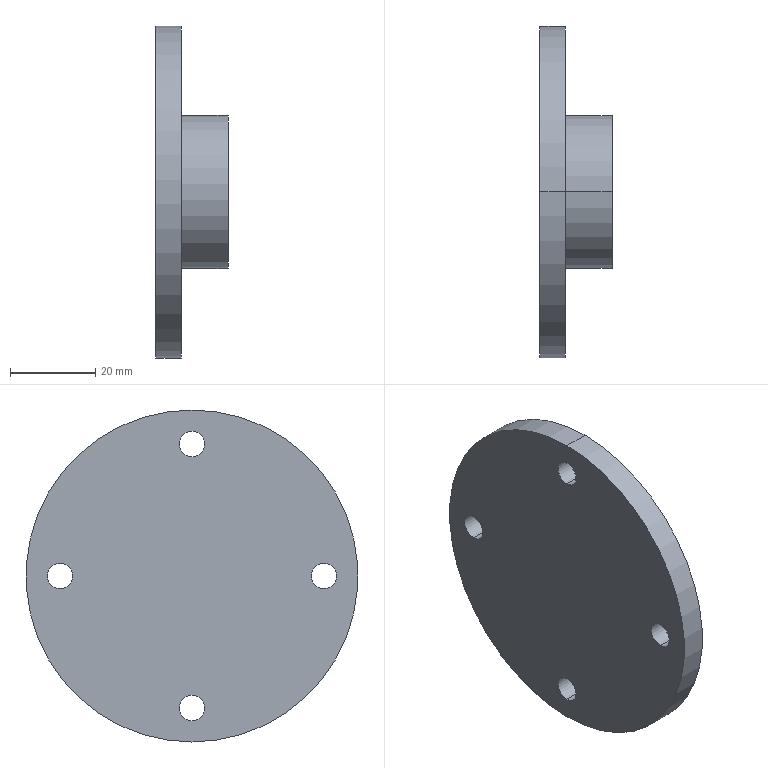Part | NX | features BREP 1 | 1 solid | 18 faces | box 17 x 78 x 78 mm | volume 32864 mm3 | cylinder 12 | plane 4 | cone 2 | commonest cylinder face diameters 6 x8 36 x2 78 x2
STEP:
#1=CARTESIAN_POINT('',(6.,0.,-28.));
#2=VERTEX_POINT('',#1);
#3=CARTESIAN_POINT('',(6.,0.,-34.));
#4=VERTEX_POINT('',#3);
#5=CARTESIAN_POINT('',(6.,0.,-31.));
#6=DIRECTION('',(1.,0.,0.));
#7=DIRECTION('',(0.,0.,1.));
#8=AXIS2_PLACEMENT_3D('',#5,#6,#7);
#9=CIRCLE('',#8,3.);
#10=EDGE_CURVE('',#2,#4,#9,.T.);
#11=ORIENTED_EDGE('',*,*,#10,.T.);
#12=CARTESIAN_POINT('',(0.,0.,-34.));
#13=VERTEX_POINT('',#12);
#14=CARTESIAN_POINT('',(17.001,0.,-34.));
#15=DIRECTION('',(-1.,0.,0.));
#16=VECTOR('',#15,1000.);
#17=LINE('',#14,#16);
#18=EDGE_CURVE('',#4,#13,#17,.T.);
#19=ORIENTED_EDGE('',*,*,#18,.T.);
#20=CARTESIAN_POINT('',(0.,0.,-28.));
#21=VERTEX_POINT('',#20);
#22=CARTESIAN_POINT('',(0.,0.,-31.));
#23=DIRECTION('',(-1.,0.,0.));
#24=DIRECTION('',(0.,0.,1.));
#25=AXIS2_PLACEMENT_3D('',#22,#23,#24);
#26=CIRCLE('',#25,3.);
#27=EDGE_CURVE('',#13,#21,#26,.T.);
#28=ORIENTED_EDGE('',*,*,#27,.T.);
#29=CARTESIAN_POINT('',(17.001,0.,-28.));
#30=DIRECTION('',(-1.,0.,0.));
#31=VECTOR('',#30,1000.);
#32=LINE('',#29,#31);
#33=EDGE_CURVE('',#2,#21,#32,.T.);
#34=ORIENTED_EDGE('',*,*,#33,.F.);
#35=EDGE_LOOP('',(#11,#19,#28,#34));
#36=FACE_BOUND('',#35,.T.);
#37=CARTESIAN_POINT('',(17.001,0.,-31.));
#38=DIRECTION('',(-1.,0.,0.));
#39=DIRECTION('',(0.,0.,-1.));
#40=AXIS2_PLACEMENT_3D('',#37,#38,#39);
#41=CYLINDRICAL_SURFACE('',#40,3.);
#42=ADVANCED_FACE('',(#36),#41,.F.);
#43=CARTESIAN_POINT('',(6.,-31.,3.));
#44=VERTEX_POINT('',#43);
#45=CARTESIAN_POINT('',(6.,-31.,-3.));
#46=VERTEX_POINT('',#45);
#47=CARTESIAN_POINT('',(6.,-31.,0.));
#48=DIRECTION('',(1.,0.,0.));
#49=DIRECTION('',(0.,0.,1.));
#50=AXIS2_PLACEMENT_3D('',#47,#48,#49);
#51=CIRCLE('',#50,3.);
#52=EDGE_CURVE('',#44,#46,#51,.T.);
#53=ORIENTED_EDGE('',*,*,#52,.T.);
#54=CARTESIAN_POINT('',(0.,-31.,-3.));
#55=VERTEX_POINT('',#54);
#56=CARTESIAN_POINT('',(17.001,-31.,-3.));
#57=DIRECTION('',(-1.,0.,0.));
#58=VECTOR('',#57,1000.);
#59=LINE('',#56,#58);
#60=EDGE_CURVE('',#46,#55,#59,.T.);
#61=ORIENTED_EDGE('',*,*,#60,.T.);
#62=CARTESIAN_POINT('',(0.,-31.,3.));
#63=VERTEX_POINT('',#62);
#64=CARTESIAN_POINT('',(0.,-31.,0.));
#65=DIRECTION('',(-1.,0.,0.));
#66=DIRECTION('',(0.,0.,1.));
#67=AXIS2_PLACEMENT_3D('',#64,#65,#66);
#68=CIRCLE('',#67,3.);
#69=EDGE_CURVE('',#55,#63,#68,.T.);
#70=ORIENTED_EDGE('',*,*,#69,.T.);
#71=CARTESIAN_POINT('',(17.001,-31.,3.));
#72=DIRECTION('',(-1.,0.,0.));
#73=VECTOR('',#72,1000.);
#74=LINE('',#71,#73);
#75=EDGE_CURVE('',#44,#63,#74,.T.);
#76=ORIENTED_EDGE('',*,*,#75,.F.);
#77=EDGE_LOOP('',(#53,#61,#70,#76));
#78=FACE_BOUND('',#77,.T.);
#79=CARTESIAN_POINT('',(17.001,-31.,0.));
#80=DIRECTION('',(-1.,0.,0.));
#81=DIRECTION('',(0.,0.,-1.));
#82=AXIS2_PLACEMENT_3D('',#79,#80,#81);
#83=CYLINDRICAL_SURFACE('',#82,3.);
#84=ADVANCED_FACE('',(#78),#83,.F.);
#85=CARTESIAN_POINT('',(6.,0.,34.));
#86=VERTEX_POINT('',#85);
#87=CARTESIAN_POINT('',(6.,0.,28.));
#88=VERTEX_POINT('',#87);
#89=CARTESIAN_POINT('',(6.,0.,31.));
#90=DIRECTION('',(1.,0.,0.));
#91=DIRECTION('',(0.,0.,1.));
#92=AXIS2_PLACEMENT_3D('',#89,#90,#91);
#93=CIRCLE('',#92,3.);
#94=EDGE_CURVE('',#86,#88,#93,.T.);
#95=ORIENTED_EDGE('',*,*,#94,.T.);
#96=CARTESIAN_POINT('',(0.,0.,28.));
#97=VERTEX_POINT('',#96);
#98=CARTESIAN_POINT('',(17.001,0.,28.));
#99=DIRECTION('',(-1.,0.,0.));
#100=VECTOR('',#99,1000.);
#101=LINE('',#98,#100);
#102=EDGE_CURVE('',#88,#97,#101,.T.);
#103=ORIENTED_EDGE('',*,*,#102,.T.);
#104=CARTESIAN_POINT('',(0.,0.,34.));
#105=VERTEX_POINT('',#104);
#106=CARTESIAN_POINT('',(0.,0.,31.));
#107=DIRECTION('',(-1.,0.,0.));
#108=DIRECTION('',(0.,0.,1.));
#109=AXIS2_PLACEMENT_3D('',#106,#107,#108);
#110=CIRCLE('',#109,3.);
#111=EDGE_CURVE('',#97,#105,#110,.T.);
#112=ORIENTED_EDGE('',*,*,#111,.T.);
#113=CARTESIAN_POINT('',(17.001,0.,34.));
#114=DIRECTION('',(-1.,0.,0.));
#115=VECTOR('',#114,1000.);
#116=LINE('',#113,#115);
#117=EDGE_CURVE('',#86,#105,#116,.T.);
#118=ORIENTED_EDGE('',*,*,#117,.F.);
#119=EDGE_LOOP('',(#95,#103,#112,#118));
#120=FACE_BOUND('',#119,.T.);
#121=CARTESIAN_POINT('',(17.001,0.,31.));
#122=DIRECTION('',(-1.,0.,0.));
#123=DIRECTION('',(0.,0.,-1.));
#124=AXIS2_PLACEMENT_3D('',#121,#122,#123);
#125=CYLINDRICAL_SURFACE('',#124,3.);
#126=ADVANCED_FACE('',(#120),#125,.F.);
#127=CARTESIAN_POINT('',(6.,31.,3.));
#128=VERTEX_POINT('',#127);
#129=CARTESIAN_POINT('',(6.,31.,-3.));
#130=VERTEX_POINT('',#129);
#131=CARTESIAN_POINT('',(6.,31.,0.));
#132=DIRECTION('',(1.,0.,0.));
#133=DIRECTION('',(0.,0.,1.));
#134=AXIS2_PLACEMENT_3D('',#131,#132,#133);
#135=CIRCLE('',#134,3.);
#136=EDGE_CURVE('',#128,#130,#135,.T.);
#137=ORIENTED_EDGE('',*,*,#136,.T.);
#138=CARTESIAN_POINT('',(0.,31.,-3.));
#139=VERTEX_POINT('',#138);
#140=CARTESIAN_POINT('',(17.001,31.,-3.));
#141=DIRECTION('',(-1.,0.,0.));
#142=VECTOR('',#141,1000.);
#143=LINE('',#140,#142);
#144=EDGE_CURVE('',#130,#139,#143,.T.);
#145=ORIENTED_EDGE('',*,*,#144,.T.);
#146=CARTESIAN_POINT('',(0.,31.,3.));
#147=VERTEX_POINT('',#146);
#148=CARTESIAN_POINT('',(0.,31.,0.));
#149=DIRECTION('',(-1.,0.,0.));
#150=DIRECTION('',(0.,0.,1.));
#151=AXIS2_PLACEMENT_3D('',#148,#149,#150);
#152=CIRCLE('',#151,3.);
#153=EDGE_CURVE('',#139,#147,#152,.T.);
#154=ORIENTED_EDGE('',*,*,#153,.T.);
#155=CARTESIAN_POINT('',(17.001,31.,3.));
#156=DIRECTION('',(-1.,0.,0.));
#157=VECTOR('',#156,1000.);
#158=LINE('',#155,#157);
#159=EDGE_CURVE('',#128,#147,#158,.T.);
#160=ORIENTED_EDGE('',*,*,#159,.F.);
#161=EDGE_LOOP('',(#137,#145,#154,#160));
#162=FACE_BOUND('',#161,.T.);
#163=CARTESIAN_POINT('',(17.001,31.,0.));
#164=DIRECTION('',(-1.,0.,0.));
#165=DIRECTION('',(0.,0.,-1.));
#166=AXIS2_PLACEMENT_3D('',#163,#164,#165);
#167=CYLINDRICAL_SURFACE('',#166,3.);
#168=ADVANCED_FACE('',(#162),#167,.F.);
#169=CARTESIAN_POINT('',(6.,0.,-12.));
#170=VERTEX_POINT('',#169);
#171=CARTESIAN_POINT('',(6.,0.,12.));
#172=VERTEX_POINT('',#171);
#173=CARTESIAN_POINT('',(6.,0.,0.));
#174=DIRECTION('',(-1.,0.,0.));
#175=DIRECTION('',(0.,0.,1.));
#176=AXIS2_PLACEMENT_3D('',#173,#174,#175);
#177=CIRCLE('',#176,12.);
#178=EDGE_CURVE('',#170,#172,#177,.T.);
#179=ORIENTED_EDGE('',*,*,#178,.T.);
#180=CARTESIAN_POINT('',(17.,0.,15.));
#181=VERTEX_POINT('',#180);
#182=CARTESIAN_POINT('',(6.,0.,12.));
#183=DIRECTION('',(0.9648,0.,0.2631));
#184=VECTOR('',#183,1000.);
#185=LINE('',#182,#184);
#186=EDGE_CURVE('',#181,#172,#185,.F.);
#187=ORIENTED_EDGE('',*,*,#186,.F.);
#188=CARTESIAN_POINT('',(17.,0.,-15.));
#189=VERTEX_POINT('',#188);
#190=CARTESIAN_POINT('',(17.,0.,0.));
#191=DIRECTION('',(-1.,0.,0.));
#192=DIRECTION('',(0.,0.,1.));
#193=AXIS2_PLACEMENT_3D('',#190,#191,#192);
#194=CIRCLE('',#193,15.);
#195=EDGE_CURVE('',#189,#181,#194,.T.);
#196=ORIENTED_EDGE('',*,*,#195,.F.);
#197=CARTESIAN_POINT('',(6.,0.,-12.));
#198=DIRECTION('',(0.9648,0.,-0.2631));
#199=VECTOR('',#198,1000.);
#200=LINE('',#197,#199);
#201=EDGE_CURVE('',#189,#170,#200,.F.);
#202=ORIENTED_EDGE('',*,*,#201,.T.);
#203=EDGE_LOOP('',(#179,#187,#196,#202));
#204=FACE_BOUND('',#203,.T.);
#205=CARTESIAN_POINT('',(6.,0.,0.));
#206=DIRECTION('',(1.,0.,0.));
#207=DIRECTION('',(0.,0.,1.));
#208=AXIS2_PLACEMENT_3D('',#205,#206,#207);
#209=CONICAL_SURFACE('',#208,12.,0.2663);
#210=ADVANCED_FACE('',(#204),#209,.F.);
#211=CARTESIAN_POINT('',(17.,0.,18.));
#212=VERTEX_POINT('',#211);
#213=CARTESIAN_POINT('',(17.,0.,-18.));
#214=VERTEX_POINT('',#213);
#215=CARTESIAN_POINT('',(17.,0.,0.));
#216=DIRECTION('',(-1.,0.,0.));
#217=DIRECTION('',(0.,0.,1.));
#218=AXIS2_PLACEMENT_3D('',#215,#216,#217);
#219=CIRCLE('',#218,18.);
#220=EDGE_CURVE('',#212,#214,#219,.T.);
#221=ORIENTED_EDGE('',*,*,#220,.T.);
#222=CARTESIAN_POINT('',(6.,0.,-18.));
#223=VERTEX_POINT('',#222);
#224=CARTESIAN_POINT('',(0.,0.,-18.));
#225=DIRECTION('',(-1.,0.,0.));
#226=VECTOR('',#225,1000.);
#227=LINE('',#224,#226);
#228=EDGE_CURVE('',#214,#223,#227,.T.);
#229=ORIENTED_EDGE('',*,*,#228,.T.);
#230=CARTESIAN_POINT('',(6.,0.,18.));
#231=VERTEX_POINT('',#230);
#232=CARTESIAN_POINT('',(6.,0.,0.));
#233=DIRECTION('',(-1.,0.,0.));
#234=DIRECTION('',(0.,0.,1.));
#235=AXIS2_PLACEMENT_3D('',#232,#233,#234);
#236=CIRCLE('',#235,18.);
#237=EDGE_CURVE('',#231,#223,#236,.T.);
#238=ORIENTED_EDGE('',*,*,#237,.F.);
#239=CARTESIAN_POINT('',(0.,0.,18.));
#240=DIRECTION('',(-1.,0.,0.));
#241=VECTOR('',#240,1000.);
#242=LINE('',#239,#241);
#243=EDGE_CURVE('',#212,#231,#242,.T.);
#244=ORIENTED_EDGE('',*,*,#243,.F.);
#245=EDGE_LOOP('',(#221,#229,#238,#244));
#246=FACE_BOUND('',#245,.T.);
#247=CARTESIAN_POINT('',(0.,0.,0.));
#248=DIRECTION('',(-1.,0.,0.));
#249=DIRECTION('',(0.,0.,-1.));
#250=AXIS2_PLACEMENT_3D('',#247,#248,#249);
#251=CYLINDRICAL_SURFACE('',#250,18.);
#252=ADVANCED_FACE('',(#246),#251,.T.);
#253=CARTESIAN_POINT('',(6.,0.,39.));
#254=VERTEX_POINT('',#253);
#255=CARTESIAN_POINT('',(6.,0.,-39.));
#256=VERTEX_POINT('',#255);
#257=CARTESIAN_POINT('',(6.,0.,0.));
#258=DIRECTION('',(-1.,0.,0.));
#259=DIRECTION('',(0.,0.,1.));
#260=AXIS2_PLACEMENT_3D('',#257,#258,#259);
#261=CIRCLE('',#260,39.);
#262=EDGE_CURVE('',#254,#256,#261,.T.);
#263=ORIENTED_EDGE('',*,*,#262,.T.);
#264=CARTESIAN_POINT('',(0.,0.,-39.));
#265=VERTEX_POINT('',#264);
#266=CARTESIAN_POINT('',(0.,0.,-39.));
#267=DIRECTION('',(-1.,0.,0.));
#268=VECTOR('',#267,1000.);
#269=LINE('',#266,#268);
#270=EDGE_CURVE('',#256,#265,#269,.T.);
#271=ORIENTED_EDGE('',*,*,#270,.T.);
#272=CARTESIAN_POINT('',(0.,0.,39.));
#273=VERTEX_POINT('',#272);
#274=CARTESIAN_POINT('',(0.,0.,0.));
#275=DIRECTION('',(-1.,0.,0.));
#276=DIRECTION('',(0.,0.,1.));
#277=AXIS2_PLACEMENT_3D('',#274,#275,#276);
#278=CIRCLE('',#277,39.);
#279=EDGE_CURVE('',#273,#265,#278,.T.);
#280=ORIENTED_EDGE('',*,*,#279,.F.);
#281=CARTESIAN_POINT('',(0.,0.,39.));
#282=DIRECTION('',(-1.,0.,0.));
#283=VECTOR('',#282,1000.);
#284=LINE('',#281,#283);
#285=EDGE_CURVE('',#254,#273,#284,.T.);
#286=ORIENTED_EDGE('',*,*,#285,.F.);
#287=EDGE_LOOP('',(#263,#271,#280,#286));
#288=FACE_BOUND('',#287,.T.);
#289=CARTESIAN_POINT('',(0.,0.,0.));
#290=DIRECTION('',(-1.,0.,0.));
#291=DIRECTION('',(0.,0.,-1.));
#292=AXIS2_PLACEMENT_3D('',#289,#290,#291);
#293=CYLINDRICAL_SURFACE('',#292,39.);
#294=ADVANCED_FACE('',(#288),#293,.T.);
#295=ORIENTED_EDGE('',*,*,#279,.T.);
#296=CARTESIAN_POINT('',(0.,0.,0.));
#297=DIRECTION('',(-1.,0.,0.));
#298=DIRECTION('',(0.,0.,1.));
#299=AXIS2_PLACEMENT_3D('',#296,#297,#298);
#300=CIRCLE('',#299,39.);
#301=EDGE_CURVE('',#265,#273,#300,.T.);
#302=ORIENTED_EDGE('',*,*,#301,.T.);
#303=EDGE_LOOP('',(#295,#302));
#304=FACE_BOUND('',#303,.T.);
#305=CARTESIAN_POINT('',(0.,0.,-31.));
#306=DIRECTION('',(-1.,0.,0.));
#307=DIRECTION('',(0.,0.,1.));
#308=AXIS2_PLACEMENT_3D('',#305,#306,#307);
#309=CIRCLE('',#308,3.);
#310=EDGE_CURVE('',#21,#13,#309,.T.);
#311=ORIENTED_EDGE('',*,*,#310,.F.);
#312=ORIENTED_EDGE('',*,*,#27,.F.);
#313=EDGE_LOOP('',(#311,#312));
#314=FACE_BOUND('',#313,.T.);
#315=CARTESIAN_POINT('',(0.,-31.,0.));
#316=DIRECTION('',(-1.,0.,0.));
#317=DIRECTION('',(0.,0.,1.));
#318=AXIS2_PLACEMENT_3D('',#315,#316,#317);
#319=CIRCLE('',#318,3.);
#320=EDGE_CURVE('',#63,#55,#319,.T.);
#321=ORIENTED_EDGE('',*,*,#320,.F.);
#322=ORIENTED_EDGE('',*,*,#69,.F.);
#323=EDGE_LOOP('',(#321,#322));
#324=FACE_BOUND('',#323,.T.);
#325=CARTESIAN_POINT('',(0.,0.,31.));
#326=DIRECTION('',(-1.,0.,0.));
#327=DIRECTION('',(0.,0.,1.));
#328=AXIS2_PLACEMENT_3D('',#325,#326,#327);
#329=CIRCLE('',#328,3.);
#330=EDGE_CURVE('',#105,#97,#329,.T.);
#331=ORIENTED_EDGE('',*,*,#330,.F.);
#332=ORIENTED_EDGE('',*,*,#111,.F.);
#333=EDGE_LOOP('',(#331,#332));
#334=FACE_BOUND('',#333,.T.);
#335=CARTESIAN_POINT('',(0.,31.,0.));
#336=DIRECTION('',(-1.,0.,0.));
#337=DIRECTION('',(0.,0.,1.));
#338=AXIS2_PLACEMENT_3D('',#335,#336,#337);
#339=CIRCLE('',#338,3.);
#340=EDGE_CURVE('',#147,#139,#339,.T.);
#341=ORIENTED_EDGE('',*,*,#340,.F.);
#342=ORIENTED_EDGE('',*,*,#153,.F.);
#343=EDGE_LOOP('',(#341,#342));
#344=FACE_BOUND('',#343,.T.);
#345=CARTESIAN_POINT('',(0.,0.,0.));
#346=DIRECTION('',(1.,0.,0.));
#347=DIRECTION('',(0.,0.,1.));
#348=AXIS2_PLACEMENT_3D('',#345,#346,#347);
#349=PLANE('',#348);
#350=ADVANCED_FACE('',(#304,#314,#324,#334,#344),#349,.F.);
#351=ORIENTED_EDGE('',*,*,#270,.F.);
#352=CARTESIAN_POINT('',(6.,0.,0.));
#353=DIRECTION('',(-1.,0.,0.));
#354=DIRECTION('',(0.,0.,1.));
#355=AXIS2_PLACEMENT_3D('',#352,#353,#354);
#356=CIRCLE('',#355,39.);
#357=EDGE_CURVE('',#256,#254,#356,.T.);
#358=ORIENTED_EDGE('',*,*,#357,.T.);
#359=ORIENTED_EDGE('',*,*,#285,.T.);
#360=ORIENTED_EDGE('',*,*,#301,.F.);
#361=EDGE_LOOP('',(#351,#358,#359,#360));
#362=FACE_BOUND('',#361,.T.);
#363=CARTESIAN_POINT('',(0.,0.,0.));
#364=DIRECTION('',(-1.,0.,0.));
#365=DIRECTION('',(0.,0.,-1.));
#366=AXIS2_PLACEMENT_3D('',#363,#364,#365);
#367=CYLINDRICAL_SURFACE('',#366,39.);
#368=ADVANCED_FACE('',(#362),#367,.T.);
#369=ORIENTED_EDGE('',*,*,#262,.F.);
#370=ORIENTED_EDGE('',*,*,#357,.F.);
#371=EDGE_LOOP('',(#369,#370));
#372=FACE_BOUND('',#371,.T.);
#373=ORIENTED_EDGE('',*,*,#10,.F.);
#374=CARTESIAN_POINT('',(6.,0.,-31.));
#375=DIRECTION('',(1.,0.,0.));
#376=DIRECTION('',(0.,0.,1.));
#377=AXIS2_PLACEMENT_3D('',#374,#375,#376);
#378=CIRCLE('',#377,3.);
#379=EDGE_CURVE('',#4,#2,#378,.T.);
#380=ORIENTED_EDGE('',*,*,#379,.F.);
#381=EDGE_LOOP('',(#373,#380));
#382=FACE_BOUND('',#381,.T.);
#383=ORIENTED_EDGE('',*,*,#52,.F.);
#384=CARTESIAN_POINT('',(6.,-31.,0.));
#385=DIRECTION('',(1.,0.,0.));
#386=DIRECTION('',(0.,0.,1.));
#387=AXIS2_PLACEMENT_3D('',#384,#385,#386);
#388=CIRCLE('',#387,3.);
#389=EDGE_CURVE('',#46,#44,#388,.T.);
#390=ORIENTED_EDGE('',*,*,#389,.F.);
#391=EDGE_LOOP('',(#383,#390));
#392=FACE_BOUND('',#391,.T.);
#393=ORIENTED_EDGE('',*,*,#94,.F.);
#394=CARTESIAN_POINT('',(6.,0.,31.));
#395=DIRECTION('',(1.,0.,0.));
#396=DIRECTION('',(0.,0.,1.));
#397=AXIS2_PLACEMENT_3D('',#394,#395,#396);
#398=CIRCLE('',#397,3.);
#399=EDGE_CURVE('',#88,#86,#398,.T.);
#400=ORIENTED_EDGE('',*,*,#399,.F.);
#401=EDGE_LOOP('',(#393,#400));
#402=FACE_BOUND('',#401,.T.);
#403=ORIENTED_EDGE('',*,*,#136,.F.);
#404=CARTESIAN_POINT('',(6.,31.,0.));
#405=DIRECTION('',(1.,0.,0.));
#406=DIRECTION('',(0.,0.,1.));
#407=AXIS2_PLACEMENT_3D('',#404,#405,#406);
#408=CIRCLE('',#407,3.);
#409=EDGE_CURVE('',#130,#128,#408,.T.);
#410=ORIENTED_EDGE('',*,*,#409,.F.);
#411=EDGE_LOOP('',(#403,#410));
#412=FACE_BOUND('',#411,.T.);
#413=ORIENTED_EDGE('',*,*,#237,.T.);
#414=CARTESIAN_POINT('',(6.,0.,0.));
#415=DIRECTION('',(-1.,0.,0.));
#416=DIRECTION('',(0.,0.,1.));
#417=AXIS2_PLACEMENT_3D('',#414,#415,#416);
#418=CIRCLE('',#417,18.);
#419=EDGE_CURVE('',#223,#231,#418,.T.);
#420=ORIENTED_EDGE('',*,*,#419,.T.);
#421=EDGE_LOOP('',(#413,#420));
#422=FACE_BOUND('',#421,.T.);
#423=CARTESIAN_POINT('',(6.,39.,0.));
#424=DIRECTION('',(-1.,0.,0.));
#425=DIRECTION('',(0.,-1.,0.));
#426=AXIS2_PLACEMENT_3D('',#423,#424,#425);
#427=PLANE('',#426);
#428=ADVANCED_FACE('',(#372,#382,#392,#402,#412,#422),#427,.F.);
#429=ORIENTED_EDGE('',*,*,#228,.F.);
#430=CARTESIAN_POINT('',(17.,0.,0.));
#431=DIRECTION('',(-1.,0.,0.));
#432=DIRECTION('',(0.,0.,1.));
#433=AXIS2_PLACEMENT_3D('',#430,#431,#432);
#434=CIRCLE('',#433,18.);
#435=EDGE_CURVE('',#214,#212,#434,.T.);
#436=ORIENTED_EDGE('',*,*,#435,.T.);
#437=ORIENTED_EDGE('',*,*,#243,.T.);
#438=ORIENTED_EDGE('',*,*,#419,.F.);
#439=EDGE_LOOP('',(#429,#436,#437,#438));
#440=FACE_BOUND('',#439,.T.);
#441=CARTESIAN_POINT('',(0.,0.,0.));
#442=DIRECTION('',(-1.,0.,0.));
#443=DIRECTION('',(0.,0.,-1.));
#444=AXIS2_PLACEMENT_3D('',#441,#442,#443);
#445=CYLINDRICAL_SURFACE('',#444,18.);
#446=ADVANCED_FACE('',(#440),#445,.T.);
#447=ORIENTED_EDGE('',*,*,#220,.F.);
#448=ORIENTED_EDGE('',*,*,#435,.F.);
#449=EDGE_LOOP('',(#447,#448));
#450=FACE_BOUND('',#449,.T.);
#451=ORIENTED_EDGE('',*,*,#195,.T.);
#452=CARTESIAN_POINT('',(17.,0.,0.));
#453=DIRECTION('',(-1.,0.,0.));
#454=DIRECTION('',(0.,0.,1.));
#455=AXIS2_PLACEMENT_3D('',#452,#453,#454);
#456=CIRCLE('',#455,15.);
#457=EDGE_CURVE('',#181,#189,#456,.T.);
#458=ORIENTED_EDGE('',*,*,#457,.T.);
#459=EDGE_LOOP('',(#451,#458));
#460=FACE_BOUND('',#459,.T.);
#461=CARTESIAN_POINT('',(17.,18.,0.));
#462=DIRECTION('',(-1.,0.,0.));
#463=DIRECTION('',(0.,-1.,0.));
#464=AXIS2_PLACEMENT_3D('',#461,#462,#463);
#465=PLANE('',#464);
#466=ADVANCED_FACE('',(#450,#460),#465,.F.);
#467=ORIENTED_EDGE('',*,*,#186,.T.);
#468=CARTESIAN_POINT('',(6.,0.,0.));
#469=DIRECTION('',(-1.,0.,0.));
#470=DIRECTION('',(0.,0.,1.));
#471=AXIS2_PLACEMENT_3D('',#468,#469,#470);
#472=CIRCLE('',#471,12.);
#473=EDGE_CURVE('',#172,#170,#472,.T.);
#474=ORIENTED_EDGE('',*,*,#473,.T.);
#475=ORIENTED_EDGE('',*,*,#201,.F.);
#476=ORIENTED_EDGE('',*,*,#457,.F.);
#477=EDGE_LOOP('',(#467,#474,#475,#476));
#478=FACE_BOUND('',#477,.T.);
#479=CARTESIAN_POINT('',(6.,0.,0.));
#480=DIRECTION('',(1.,0.,0.));
#481=DIRECTION('',(0.,0.,1.));
#482=AXIS2_PLACEMENT_3D('',#479,#480,#481);
#483=CONICAL_SURFACE('',#482,12.,0.2663);
#484=ADVANCED_FACE('',(#478),#483,.F.);
#485=ORIENTED_EDGE('',*,*,#178,.F.);
#486=ORIENTED_EDGE('',*,*,#473,.F.);
#487=EDGE_LOOP('',(#485,#486));
#488=FACE_BOUND('',#487,.T.);
#489=CARTESIAN_POINT('',(6.,12.,0.));
#490=DIRECTION('',(-1.,0.,0.));
#491=DIRECTION('',(0.,-1.,0.));
#492=AXIS2_PLACEMENT_3D('',#489,#490,#491);
#493=PLANE('',#492);
#494=ADVANCED_FACE('',(#488),#493,.F.);
#495=ORIENTED_EDGE('',*,*,#144,.F.);
#496=ORIENTED_EDGE('',*,*,#409,.T.);
#497=ORIENTED_EDGE('',*,*,#159,.T.);
#498=ORIENTED_EDGE('',*,*,#340,.T.);
#499=EDGE_LOOP('',(#495,#496,#497,#498));
#500=FACE_BOUND('',#499,.T.);
#501=CARTESIAN_POINT('',(17.001,31.,0.));
#502=DIRECTION('',(-1.,0.,0.));
#503=DIRECTION('',(0.,0.,-1.));
#504=AXIS2_PLACEMENT_3D('',#501,#502,#503);
#505=CYLINDRICAL_SURFACE('',#504,3.);
#506=ADVANCED_FACE('',(#500),#505,.F.);
#507=ORIENTED_EDGE('',*,*,#102,.F.);
#508=ORIENTED_EDGE('',*,*,#399,.T.);
#509=ORIENTED_EDGE('',*,*,#117,.T.);
#510=ORIENTED_EDGE('',*,*,#330,.T.);
#511=EDGE_LOOP('',(#507,#508,#509,#510));
#512=FACE_BOUND('',#511,.T.);
#513=CARTESIAN_POINT('',(17.001,0.,31.));
#514=DIRECTION('',(-1.,0.,0.));
#515=DIRECTION('',(0.,0.,-1.));
#516=AXIS2_PLACEMENT_3D('',#513,#514,#515);
#517=CYLINDRICAL_SURFACE('',#516,3.);
#518=ADVANCED_FACE('',(#512),#517,.F.);
#519=ORIENTED_EDGE('',*,*,#60,.F.);
#520=ORIENTED_EDGE('',*,*,#389,.T.);
#521=ORIENTED_EDGE('',*,*,#75,.T.);
#522=ORIENTED_EDGE('',*,*,#320,.T.);
#523=EDGE_LOOP('',(#519,#520,#521,#522));
#524=FACE_BOUND('',#523,.T.);
#525=CARTESIAN_POINT('',(17.001,-31.,0.));
#526=DIRECTION('',(-1.,0.,0.));
#527=DIRECTION('',(0.,0.,-1.));
#528=AXIS2_PLACEMENT_3D('',#525,#526,#527);
#529=CYLINDRICAL_SURFACE('',#528,3.);
#530=ADVANCED_FACE('',(#524),#529,.F.);
#531=ORIENTED_EDGE('',*,*,#18,.F.);
#532=ORIENTED_EDGE('',*,*,#379,.T.);
#533=ORIENTED_EDGE('',*,*,#33,.T.);
#534=ORIENTED_EDGE('',*,*,#310,.T.);
#535=EDGE_LOOP('',(#531,#532,#533,#534));
#536=FACE_BOUND('',#535,.T.);
#537=CARTESIAN_POINT('',(17.001,0.,-31.));
#538=DIRECTION('',(-1.,0.,0.));
#539=DIRECTION('',(0.,0.,-1.));
#540=AXIS2_PLACEMENT_3D('',#537,#538,#539);
#541=CYLINDRICAL_SURFACE('',#540,3.);
#542=ADVANCED_FACE('',(#536),#541,.F.);
#543=CLOSED_SHELL('',(#42,#84,#126,#168,#210,#252,#294,#350,#368,#428,#446,#466,#484,#494,#506,#518,#530,#542));
#544=MANIFOLD_SOLID_BREP('',#543);
#545=(LENGTH_UNIT()NAMED_UNIT(*)SI_UNIT(.MILLI.,.METRE.));
#546=UNCERTAINTY_MEASURE_WITH_UNIT(LENGTH_MEASURE(0.00001),#545,'','');
#547=(NAMED_UNIT(*)PLANE_ANGLE_UNIT()SI_UNIT($,.RADIAN.));
#548=(NAMED_UNIT(*)SI_UNIT($,.STERADIAN.)SOLID_ANGLE_UNIT());
#549=(GEOMETRIC_REPRESENTATION_CONTEXT(3)GLOBAL_UNCERTAINTY_ASSIGNED_CONTEXT((#546))GLOBAL_UNIT_ASSIGNED_CONTEXT((#545,#547,#548))REPRESENTATION_CONTEXT('',''));
#550=ADVANCED_BREP_SHAPE_REPRESENTATION('',(#544),#549);